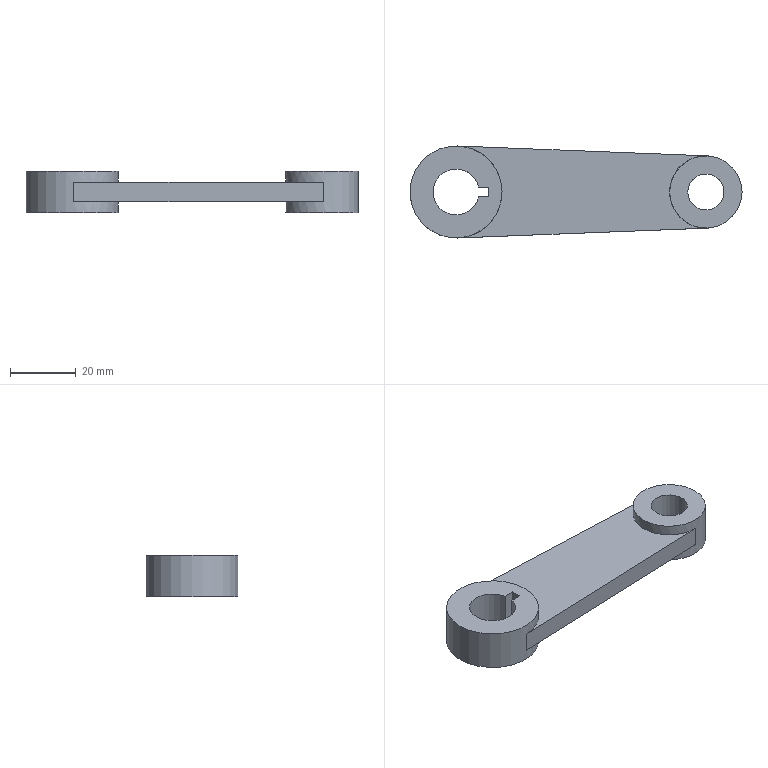Part | NX | features EXTRUDE 3, DATUM_CSYS 2, SKETCH 1 | 1 solid | 15 faces | box 101 x 28 x 12.5 mm | volume 17643 mm3 | plane 11 | cylinder 4 | commonest cylinder face diameters 11 x1 14 x1 22 x1 28 x1
STEP:
#1=CARTESIAN_POINT('',(14.,0.,-6.25));
#2=VERTEX_POINT('',#1);
#3=CARTESIAN_POINT('',(0.,0.,-6.25));
#4=DIRECTION('',(0.,0.,1.));
#5=DIRECTION('',(1.,0.,0.));
#6=AXIS2_PLACEMENT_3D('',#3,#4,#5);
#7=CIRCLE('',#6,14.);
#8=EDGE_CURVE('',#2,#2,#7,.T.);
#9=ORIENTED_EDGE('',*,*,#8,.T.);
#10=EDGE_LOOP('',(#9));
#11=FACE_BOUND('',#10,.T.);
#12=CARTESIAN_POINT('',(14.,0.,6.25));
#13=VERTEX_POINT('',#12);
#14=CARTESIAN_POINT('',(0.,0.,6.25));
#15=DIRECTION('',(0.,0.,1.));
#16=DIRECTION('',(1.,0.,0.));
#17=AXIS2_PLACEMENT_3D('',#14,#15,#16);
#18=CIRCLE('',#17,14.);
#19=EDGE_CURVE('',#13,#13,#18,.T.);
#20=ORIENTED_EDGE('',*,*,#19,.F.);
#21=EDGE_LOOP('',(#20));
#22=FACE_BOUND('',#21,.T.);
#23=CARTESIAN_POINT('',(0.5526,-13.989,3.));
#24=VERTEX_POINT('',#23);
#25=CARTESIAN_POINT('',(0.5526,-13.989,-3.));
#26=VERTEX_POINT('',#25);
#27=CARTESIAN_POINT('',(0.5526,-13.989,3.));
#28=DIRECTION('',(0.,0.,-1.));
#29=VECTOR('',#28,1000.);
#30=LINE('',#27,#29);
#31=EDGE_CURVE('',#24,#26,#30,.T.);
#32=ORIENTED_EDGE('',*,*,#31,.F.);
#33=CARTESIAN_POINT('',(0.5526,13.989,3.));
#34=VERTEX_POINT('',#33);
#35=CARTESIAN_POINT('',(0.,0.,3.));
#36=DIRECTION('',(0.,0.,-1.));
#37=DIRECTION('',(1.,0.,0.));
#38=AXIS2_PLACEMENT_3D('',#35,#36,#37);
#39=CIRCLE('',#38,14.);
#40=EDGE_CURVE('',#34,#24,#39,.T.);
#41=ORIENTED_EDGE('',*,*,#40,.F.);
#42=CARTESIAN_POINT('',(0.5526,13.989,-3.));
#43=VERTEX_POINT('',#42);
#44=CARTESIAN_POINT('',(0.5526,13.989,3.));
#45=DIRECTION('',(0.,0.,-1.));
#46=VECTOR('',#45,1000.);
#47=LINE('',#44,#46);
#48=EDGE_CURVE('',#34,#43,#47,.T.);
#49=ORIENTED_EDGE('',*,*,#48,.T.);
#50=CARTESIAN_POINT('',(0.,0.,-3.));
#51=DIRECTION('',(0.,0.,-1.));
#52=DIRECTION('',(1.,0.,0.));
#53=AXIS2_PLACEMENT_3D('',#50,#51,#52);
#54=CIRCLE('',#53,14.);
#55=EDGE_CURVE('',#43,#26,#54,.T.);
#56=ORIENTED_EDGE('',*,*,#55,.T.);
#57=EDGE_LOOP('',(#32,#41,#49,#56));
#58=FACE_BOUND('',#57,.T.);
#59=CARTESIAN_POINT('',(0.,0.,6.25));
#60=DIRECTION('',(0.,0.,-1.));
#61=DIRECTION('',(-1.,0.,0.));
#62=AXIS2_PLACEMENT_3D('',#59,#60,#61);
#63=CYLINDRICAL_SURFACE('',#62,14.);
#64=ADVANCED_FACE('',(#11,#22,#58),#63,.T.);
#65=CARTESIAN_POINT('',(6.837,-1.5,-6.25));
#66=VERTEX_POINT('',#65);
#67=CARTESIAN_POINT('',(6.837,1.5,-6.25));
#68=VERTEX_POINT('',#67);
#69=CARTESIAN_POINT('',(0.,0.,-6.25));
#70=DIRECTION('',(0.,0.,-1.));
#71=DIRECTION('',(1.,0.,0.));
#72=AXIS2_PLACEMENT_3D('',#69,#70,#71);
#73=CIRCLE('',#72,7.);
#74=EDGE_CURVE('',#66,#68,#73,.T.);
#75=ORIENTED_EDGE('',*,*,#74,.T.);
#76=CARTESIAN_POINT('',(6.837,1.5,6.25));
#77=VERTEX_POINT('',#76);
#78=CARTESIAN_POINT('',(6.837,1.5,6.25));
#79=DIRECTION('',(0.,0.,-1.));
#80=VECTOR('',#79,1000.);
#81=LINE('',#78,#80);
#82=EDGE_CURVE('',#77,#68,#81,.T.);
#83=ORIENTED_EDGE('',*,*,#82,.F.);
#84=CARTESIAN_POINT('',(6.837,-1.5,6.25));
#85=VERTEX_POINT('',#84);
#86=CARTESIAN_POINT('',(0.,0.,6.25));
#87=DIRECTION('',(0.,0.,-1.));
#88=DIRECTION('',(1.,0.,0.));
#89=AXIS2_PLACEMENT_3D('',#86,#87,#88);
#90=CIRCLE('',#89,7.);
#91=EDGE_CURVE('',#85,#77,#90,.T.);
#92=ORIENTED_EDGE('',*,*,#91,.F.);
#93=CARTESIAN_POINT('',(6.837,-1.5,6.25));
#94=DIRECTION('',(0.,0.,-1.));
#95=VECTOR('',#94,1000.);
#96=LINE('',#93,#95);
#97=EDGE_CURVE('',#85,#66,#96,.T.);
#98=ORIENTED_EDGE('',*,*,#97,.T.);
#99=EDGE_LOOP('',(#75,#83,#92,#98));
#100=FACE_BOUND('',#99,.T.);
#101=CARTESIAN_POINT('',(0.,0.,6.25));
#102=DIRECTION('',(0.,0.,-1.));
#103=DIRECTION('',(-1.,0.,0.));
#104=AXIS2_PLACEMENT_3D('',#101,#102,#103);
#105=CYLINDRICAL_SURFACE('',#104,7.);
#106=ADVANCED_FACE('',(#100),#105,.F.);
#107=CARTESIAN_POINT('',(10.,1.5,-6.25));
#108=VERTEX_POINT('',#107);
#109=CARTESIAN_POINT('',(6.837,1.5,-6.25));
#110=DIRECTION('',(1.,0.,0.));
#111=VECTOR('',#110,1000.);
#112=LINE('',#109,#111);
#113=EDGE_CURVE('',#68,#108,#112,.T.);
#114=ORIENTED_EDGE('',*,*,#113,.T.);
#115=CARTESIAN_POINT('',(10.,1.5,6.25));
#116=VERTEX_POINT('',#115);
#117=CARTESIAN_POINT('',(10.,1.5,6.25));
#118=DIRECTION('',(0.,0.,-1.));
#119=VECTOR('',#118,1000.);
#120=LINE('',#117,#119);
#121=EDGE_CURVE('',#116,#108,#120,.T.);
#122=ORIENTED_EDGE('',*,*,#121,.F.);
#123=CARTESIAN_POINT('',(6.837,1.5,6.25));
#124=DIRECTION('',(1.,0.,0.));
#125=VECTOR('',#124,1000.);
#126=LINE('',#123,#125);
#127=EDGE_CURVE('',#77,#116,#126,.T.);
#128=ORIENTED_EDGE('',*,*,#127,.F.);
#129=ORIENTED_EDGE('',*,*,#82,.T.);
#130=EDGE_LOOP('',(#114,#122,#128,#129));
#131=FACE_BOUND('',#130,.T.);
#132=CARTESIAN_POINT('',(6.837,1.5,6.25));
#133=DIRECTION('',(0.,1.,0.));
#134=DIRECTION('',(-1.,0.,0.));
#135=AXIS2_PLACEMENT_3D('',#132,#133,#134);
#136=PLANE('',#135);
#137=ADVANCED_FACE('',(#131),#136,.F.);
#138=CARTESIAN_POINT('',(10.,-1.5,-6.25));
#139=VERTEX_POINT('',#138);
#140=CARTESIAN_POINT('',(10.,1.5,-6.25));
#141=DIRECTION('',(0.,-1.,0.));
#142=VECTOR('',#141,1000.);
#143=LINE('',#140,#142);
#144=EDGE_CURVE('',#108,#139,#143,.T.);
#145=ORIENTED_EDGE('',*,*,#144,.T.);
#146=CARTESIAN_POINT('',(10.,-1.5,6.25));
#147=VERTEX_POINT('',#146);
#148=CARTESIAN_POINT('',(10.,-1.5,6.25));
#149=DIRECTION('',(0.,0.,-1.));
#150=VECTOR('',#149,1000.);
#151=LINE('',#148,#150);
#152=EDGE_CURVE('',#147,#139,#151,.T.);
#153=ORIENTED_EDGE('',*,*,#152,.F.);
#154=CARTESIAN_POINT('',(10.,1.5,6.25));
#155=DIRECTION('',(0.,-1.,0.));
#156=VECTOR('',#155,1000.);
#157=LINE('',#154,#156);
#158=EDGE_CURVE('',#116,#147,#157,.T.);
#159=ORIENTED_EDGE('',*,*,#158,.F.);
#160=ORIENTED_EDGE('',*,*,#121,.T.);
#161=EDGE_LOOP('',(#145,#153,#159,#160));
#162=FACE_BOUND('',#161,.T.);
#163=CARTESIAN_POINT('',(10.,1.5,6.25));
#164=DIRECTION('',(1.,0.,0.));
#165=DIRECTION('',(0.,0.,-1.));
#166=AXIS2_PLACEMENT_3D('',#163,#164,#165);
#167=PLANE('',#166);
#168=ADVANCED_FACE('',(#162),#167,.F.);
#169=CARTESIAN_POINT('',(10.,-1.5,-6.25));
#170=DIRECTION('',(-1.,0.,0.));
#171=VECTOR('',#170,1000.);
#172=LINE('',#169,#171);
#173=EDGE_CURVE('',#139,#66,#172,.T.);
#174=ORIENTED_EDGE('',*,*,#173,.T.);
#175=ORIENTED_EDGE('',*,*,#97,.F.);
#176=CARTESIAN_POINT('',(10.,-1.5,6.25));
#177=DIRECTION('',(-1.,0.,0.));
#178=VECTOR('',#177,1000.);
#179=LINE('',#176,#178);
#180=EDGE_CURVE('',#147,#85,#179,.T.);
#181=ORIENTED_EDGE('',*,*,#180,.F.);
#182=ORIENTED_EDGE('',*,*,#152,.T.);
#183=EDGE_LOOP('',(#174,#175,#181,#182));
#184=FACE_BOUND('',#183,.T.);
#185=CARTESIAN_POINT('',(10.,-1.5,6.25));
#186=DIRECTION('',(0.,-1.,0.));
#187=DIRECTION('',(1.,0.,0.));
#188=AXIS2_PLACEMENT_3D('',#185,#186,#187);
#189=PLANE('',#188);
#190=ADVANCED_FACE('',(#184),#189,.F.);
#191=ORIENTED_EDGE('',*,*,#19,.T.);
#192=EDGE_LOOP('',(#191));
#193=FACE_BOUND('',#192,.T.);
#194=ORIENTED_EDGE('',*,*,#91,.T.);
#195=ORIENTED_EDGE('',*,*,#127,.T.);
#196=ORIENTED_EDGE('',*,*,#158,.T.);
#197=ORIENTED_EDGE('',*,*,#180,.T.);
#198=EDGE_LOOP('',(#194,#195,#196,#197));
#199=FACE_BOUND('',#198,.T.);
#200=CARTESIAN_POINT('',(0.,0.,6.25));
#201=DIRECTION('',(0.,0.,1.));
#202=DIRECTION('',(1.,0.,0.));
#203=AXIS2_PLACEMENT_3D('',#200,#201,#202);
#204=PLANE('',#203);
#205=ADVANCED_FACE('',(#193,#199),#204,.T.);
#206=ORIENTED_EDGE('',*,*,#8,.F.);
#207=EDGE_LOOP('',(#206));
#208=FACE_BOUND('',#207,.T.);
#209=ORIENTED_EDGE('',*,*,#74,.F.);
#210=ORIENTED_EDGE('',*,*,#173,.F.);
#211=ORIENTED_EDGE('',*,*,#144,.F.);
#212=ORIENTED_EDGE('',*,*,#113,.F.);
#213=EDGE_LOOP('',(#209,#210,#211,#212));
#214=FACE_BOUND('',#213,.T.);
#215=CARTESIAN_POINT('',(0.,0.,-6.25));
#216=DIRECTION('',(0.,0.,1.));
#217=DIRECTION('',(1.,0.,0.));
#218=AXIS2_PLACEMENT_3D('',#215,#216,#217);
#219=PLANE('',#218);
#220=ADVANCED_FACE('',(#208,#214),#219,.F.);
#221=CARTESIAN_POINT('',(76.434,-10.991,-3.));
#222=VERTEX_POINT('',#221);
#223=CARTESIAN_POINT('',(0.5526,-13.989,-3.));
#224=DIRECTION('',(0.9992,0.03947,0.));
#225=VECTOR('',#224,1000.);
#226=LINE('',#223,#225);
#227=EDGE_CURVE('',#26,#222,#226,.T.);
#228=ORIENTED_EDGE('',*,*,#227,.T.);
#229=CARTESIAN_POINT('',(76.434,-10.991,3.));
#230=VERTEX_POINT('',#229);
#231=CARTESIAN_POINT('',(76.434,-10.991,3.));
#232=DIRECTION('',(0.,0.,-1.));
#233=VECTOR('',#232,1000.);
#234=LINE('',#231,#233);
#235=EDGE_CURVE('',#230,#222,#234,.T.);
#236=ORIENTED_EDGE('',*,*,#235,.F.);
#237=CARTESIAN_POINT('',(0.5526,-13.989,3.));
#238=DIRECTION('',(0.9992,0.03947,0.));
#239=VECTOR('',#238,1000.);
#240=LINE('',#237,#239);
#241=EDGE_CURVE('',#24,#230,#240,.T.);
#242=ORIENTED_EDGE('',*,*,#241,.F.);
#243=ORIENTED_EDGE('',*,*,#31,.T.);
#244=EDGE_LOOP('',(#228,#236,#242,#243));
#245=FACE_BOUND('',#244,.T.);
#246=CARTESIAN_POINT('',(0.5526,-13.989,3.));
#247=DIRECTION('',(-0.03947,0.9992,0.));
#248=DIRECTION('',(-0.9992,-0.03947,0.));
#249=AXIS2_PLACEMENT_3D('',#246,#247,#248);
#250=PLANE('',#249);
#251=ADVANCED_FACE('',(#245),#250,.F.);
#252=CARTESIAN_POINT('',(76.434,10.991,-3.));
#253=VERTEX_POINT('',#252);
#254=CARTESIAN_POINT('',(76.434,10.991,-3.));
#255=DIRECTION('',(-0.9992,0.03947,0.));
#256=VECTOR('',#255,1000.);
#257=LINE('',#254,#256);
#258=EDGE_CURVE('',#253,#43,#257,.T.);
#259=ORIENTED_EDGE('',*,*,#258,.T.);
#260=ORIENTED_EDGE('',*,*,#48,.F.);
#261=CARTESIAN_POINT('',(76.434,10.991,3.));
#262=VERTEX_POINT('',#261);
#263=CARTESIAN_POINT('',(76.434,10.991,3.));
#264=DIRECTION('',(-0.9992,0.03947,0.));
#265=VECTOR('',#264,1000.);
#266=LINE('',#263,#265);
#267=EDGE_CURVE('',#262,#34,#266,.T.);
#268=ORIENTED_EDGE('',*,*,#267,.F.);
#269=CARTESIAN_POINT('',(76.434,10.991,3.));
#270=DIRECTION('',(0.,0.,-1.));
#271=VECTOR('',#270,1000.);
#272=LINE('',#269,#271);
#273=EDGE_CURVE('',#262,#253,#272,.T.);
#274=ORIENTED_EDGE('',*,*,#273,.T.);
#275=EDGE_LOOP('',(#259,#260,#268,#274));
#276=FACE_BOUND('',#275,.T.);
#277=CARTESIAN_POINT('',(76.434,10.991,3.));
#278=DIRECTION('',(-0.03947,-0.9992,0.));
#279=DIRECTION('',(0.9992,-0.03947,0.));
#280=AXIS2_PLACEMENT_3D('',#277,#278,#279);
#281=PLANE('',#280);
#282=ADVANCED_FACE('',(#276),#281,.F.);
#283=ORIENTED_EDGE('',*,*,#40,.T.);
#284=ORIENTED_EDGE('',*,*,#241,.T.);
#285=CARTESIAN_POINT('',(76.,0.,3.));
#286=DIRECTION('',(0.,0.,-1.));
#287=DIRECTION('',(1.,0.,0.));
#288=AXIS2_PLACEMENT_3D('',#285,#286,#287);
#289=CIRCLE('',#288,11.);
#290=EDGE_CURVE('',#230,#262,#289,.T.);
#291=ORIENTED_EDGE('',*,*,#290,.T.);
#292=ORIENTED_EDGE('',*,*,#267,.T.);
#293=EDGE_LOOP('',(#283,#284,#291,#292));
#294=FACE_BOUND('',#293,.T.);
#295=CARTESIAN_POINT('',(0.,0.,3.));
#296=DIRECTION('',(0.,0.,-1.));
#297=DIRECTION('',(-1.,0.,0.));
#298=AXIS2_PLACEMENT_3D('',#295,#296,#297);
#299=PLANE('',#298);
#300=ADVANCED_FACE('',(#294),#299,.F.);
#301=ORIENTED_EDGE('',*,*,#55,.F.);
#302=ORIENTED_EDGE('',*,*,#258,.F.);
#303=CARTESIAN_POINT('',(76.,0.,-3.));
#304=DIRECTION('',(0.,0.,-1.));
#305=DIRECTION('',(1.,0.,0.));
#306=AXIS2_PLACEMENT_3D('',#303,#304,#305);
#307=CIRCLE('',#306,11.);
#308=EDGE_CURVE('',#222,#253,#307,.T.);
#309=ORIENTED_EDGE('',*,*,#308,.F.);
#310=ORIENTED_EDGE('',*,*,#227,.F.);
#311=EDGE_LOOP('',(#301,#302,#309,#310));
#312=FACE_BOUND('',#311,.T.);
#313=CARTESIAN_POINT('',(0.,0.,-3.));
#314=DIRECTION('',(0.,0.,-1.));
#315=DIRECTION('',(-1.,0.,0.));
#316=AXIS2_PLACEMENT_3D('',#313,#314,#315);
#317=PLANE('',#316);
#318=ADVANCED_FACE('',(#312),#317,.T.);
#319=ORIENTED_EDGE('',*,*,#273,.F.);
#320=ORIENTED_EDGE('',*,*,#290,.F.);
#321=ORIENTED_EDGE('',*,*,#235,.T.);
#322=ORIENTED_EDGE('',*,*,#308,.T.);
#323=EDGE_LOOP('',(#319,#320,#321,#322));
#324=FACE_BOUND('',#323,.T.);
#325=CARTESIAN_POINT('',(87.,0.,6.25));
#326=VERTEX_POINT('',#325);
#327=CARTESIAN_POINT('',(76.,0.,6.25));
#328=DIRECTION('',(0.,0.,1.));
#329=DIRECTION('',(1.,0.,0.));
#330=AXIS2_PLACEMENT_3D('',#327,#328,#329);
#331=CIRCLE('',#330,11.);
#332=EDGE_CURVE('',#326,#326,#331,.T.);
#333=ORIENTED_EDGE('',*,*,#332,.F.);
#334=EDGE_LOOP('',(#333));
#335=FACE_BOUND('',#334,.T.);
#336=CARTESIAN_POINT('',(87.,0.,-6.25));
#337=VERTEX_POINT('',#336);
#338=CARTESIAN_POINT('',(76.,0.,-6.25));
#339=DIRECTION('',(0.,0.,1.));
#340=DIRECTION('',(1.,0.,0.));
#341=AXIS2_PLACEMENT_3D('',#338,#339,#340);
#342=CIRCLE('',#341,11.);
#343=EDGE_CURVE('',#337,#337,#342,.T.);
#344=ORIENTED_EDGE('',*,*,#343,.T.);
#345=EDGE_LOOP('',(#344));
#346=FACE_BOUND('',#345,.T.);
#347=CARTESIAN_POINT('',(76.,0.,6.25));
#348=DIRECTION('',(0.,0.,-1.));
#349=DIRECTION('',(-1.,0.,0.));
#350=AXIS2_PLACEMENT_3D('',#347,#348,#349);
#351=CYLINDRICAL_SURFACE('',#350,11.);
#352=ADVANCED_FACE('',(#324,#335,#346),#351,.T.);
#353=CARTESIAN_POINT('',(81.5,0.,6.25));
#354=VERTEX_POINT('',#353);
#355=CARTESIAN_POINT('',(76.,0.,6.25));
#356=DIRECTION('',(0.,0.,1.));
#357=DIRECTION('',(1.,0.,0.));
#358=AXIS2_PLACEMENT_3D('',#355,#356,#357);
#359=CIRCLE('',#358,5.5);
#360=EDGE_CURVE('',#354,#354,#359,.T.);
#361=ORIENTED_EDGE('',*,*,#360,.T.);
#362=EDGE_LOOP('',(#361));
#363=FACE_BOUND('',#362,.T.);
#364=CARTESIAN_POINT('',(81.5,0.,-6.25));
#365=VERTEX_POINT('',#364);
#366=CARTESIAN_POINT('',(76.,0.,-6.25));
#367=DIRECTION('',(0.,0.,1.));
#368=DIRECTION('',(1.,0.,0.));
#369=AXIS2_PLACEMENT_3D('',#366,#367,#368);
#370=CIRCLE('',#369,5.5);
#371=EDGE_CURVE('',#365,#365,#370,.T.);
#372=ORIENTED_EDGE('',*,*,#371,.F.);
#373=EDGE_LOOP('',(#372));
#374=FACE_BOUND('',#373,.T.);
#375=CARTESIAN_POINT('',(76.,0.,6.25));
#376=DIRECTION('',(0.,0.,-1.));
#377=DIRECTION('',(-1.,0.,0.));
#378=AXIS2_PLACEMENT_3D('',#375,#376,#377);
#379=CYLINDRICAL_SURFACE('',#378,5.5);
#380=ADVANCED_FACE('',(#363,#374),#379,.F.);
#381=ORIENTED_EDGE('',*,*,#332,.T.);
#382=EDGE_LOOP('',(#381));
#383=FACE_BOUND('',#382,.T.);
#384=ORIENTED_EDGE('',*,*,#360,.F.);
#385=EDGE_LOOP('',(#384));
#386=FACE_BOUND('',#385,.T.);
#387=CARTESIAN_POINT('',(76.,0.,6.25));
#388=DIRECTION('',(0.,0.,1.));
#389=DIRECTION('',(1.,0.,0.));
#390=AXIS2_PLACEMENT_3D('',#387,#388,#389);
#391=PLANE('',#390);
#392=ADVANCED_FACE('',(#383,#386),#391,.T.);
#393=ORIENTED_EDGE('',*,*,#343,.F.);
#394=EDGE_LOOP('',(#393));
#395=FACE_BOUND('',#394,.T.);
#396=ORIENTED_EDGE('',*,*,#371,.T.);
#397=EDGE_LOOP('',(#396));
#398=FACE_BOUND('',#397,.T.);
#399=CARTESIAN_POINT('',(76.,0.,-6.25));
#400=DIRECTION('',(0.,0.,1.));
#401=DIRECTION('',(1.,0.,0.));
#402=AXIS2_PLACEMENT_3D('',#399,#400,#401);
#403=PLANE('',#402);
#404=ADVANCED_FACE('',(#395,#398),#403,.F.);
#405=CLOSED_SHELL('',(#64,#106,#137,#168,#190,#205,#220,#251,#282,#300,#318,#352,#380,#392,#404));
#406=MANIFOLD_SOLID_BREP('',#405);
#407=(LENGTH_UNIT()NAMED_UNIT(*)SI_UNIT(.MILLI.,.METRE.));
#408=UNCERTAINTY_MEASURE_WITH_UNIT(LENGTH_MEASURE(0.00001),#407,'','');
#409=(NAMED_UNIT(*)PLANE_ANGLE_UNIT()SI_UNIT($,.RADIAN.));
#410=(NAMED_UNIT(*)SI_UNIT($,.STERADIAN.)SOLID_ANGLE_UNIT());
#411=(GEOMETRIC_REPRESENTATION_CONTEXT(3)GLOBAL_UNCERTAINTY_ASSIGNED_CONTEXT((#408))GLOBAL_UNIT_ASSIGNED_CONTEXT((#407,#409,#410))REPRESENTATION_CONTEXT('',''));
#412=ADVANCED_BREP_SHAPE_REPRESENTATION('',(#406),#411);